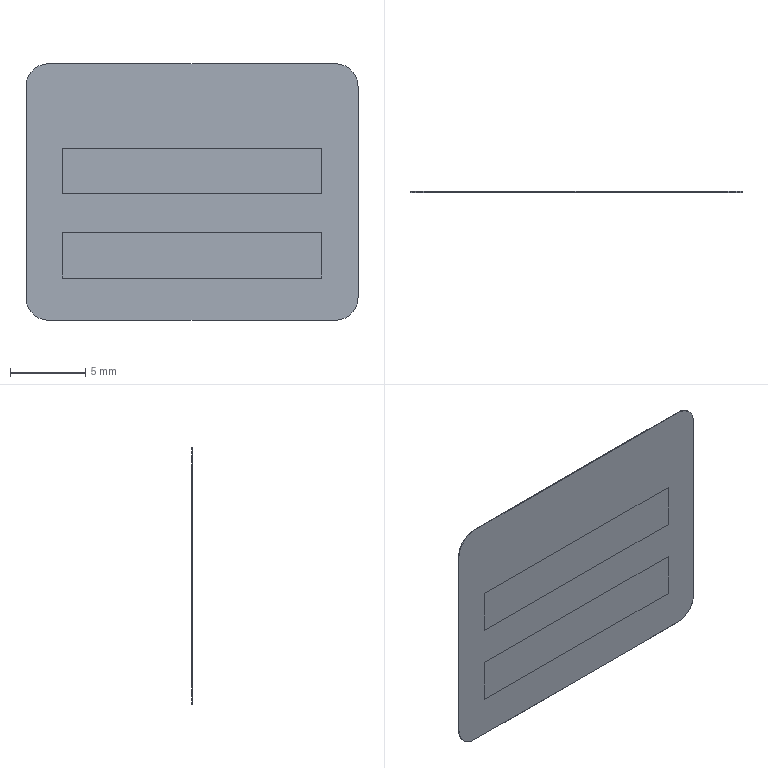Part | NX | features BREP 1 | 1 solid | 12 faces | box 22 x 0.06 x 17 mm | volume 18.947 mm3 | plane 8 | cylinder 4 | commonest cylinder face diameters 3 x4
STEP:
#1=CARTESIAN_POINT('',(2.4,-0.005,2.8));
#2=VERTEX_POINT('',#1);
#3=CARTESIAN_POINT('',(19.6,-0.005,2.8));
#4=VERTEX_POINT('',#3);
#5=CARTESIAN_POINT('',(2.4,-0.01,2.8));
#6=CARTESIAN_POINT('',(8.133,-0.01,2.8));
#7=CARTESIAN_POINT('',(13.867,-0.01,2.8));
#8=CARTESIAN_POINT('',(19.6,-0.01,2.8));
#9=B_SPLINE_CURVE_WITH_KNOTS('',3,(#5,#6,#7,#8),.UNSPECIFIED.,.F.,.F.,(4,4),(0.,1.),.UNSPECIFIED.);
#10=EDGE_CURVE('',#2,#4,#9,.T.);
#11=ORIENTED_EDGE('',*,*,#10,.T.);
#12=CARTESIAN_POINT('',(19.6,-0.005,5.8));
#13=VERTEX_POINT('',#12);
#14=CARTESIAN_POINT('',(19.6,-0.01,2.8));
#15=CARTESIAN_POINT('',(19.6,-0.01,3.8));
#16=CARTESIAN_POINT('',(19.6,-0.01,4.8));
#17=CARTESIAN_POINT('',(19.6,-0.01,5.8));
#18=B_SPLINE_CURVE_WITH_KNOTS('',3,(#14,#15,#16,#17),.UNSPECIFIED.,.F.,.F.,(4,4),(0.,1.),.UNSPECIFIED.);
#19=EDGE_CURVE('',#4,#13,#18,.T.);
#20=ORIENTED_EDGE('',*,*,#19,.T.);
#21=CARTESIAN_POINT('',(2.4,-0.005,5.8));
#22=VERTEX_POINT('',#21);
#23=CARTESIAN_POINT('',(19.6,-0.01,5.8));
#24=CARTESIAN_POINT('',(13.867,-0.01,5.8));
#25=CARTESIAN_POINT('',(8.133,-0.01,5.8));
#26=CARTESIAN_POINT('',(2.4,-0.01,5.8));
#27=B_SPLINE_CURVE_WITH_KNOTS('',3,(#23,#24,#25,#26),.UNSPECIFIED.,.F.,.F.,(4,4),(0.,1.),.UNSPECIFIED.);
#28=EDGE_CURVE('',#13,#22,#27,.T.);
#29=ORIENTED_EDGE('',*,*,#28,.T.);
#30=CARTESIAN_POINT('',(2.4,-0.01,5.8));
#31=CARTESIAN_POINT('',(2.4,-0.01,4.8));
#32=CARTESIAN_POINT('',(2.4,-0.01,3.8));
#33=CARTESIAN_POINT('',(2.4,-0.01,2.8));
#34=B_SPLINE_CURVE_WITH_KNOTS('',3,(#30,#31,#32,#33),.UNSPECIFIED.,.F.,.F.,(4,4),(0.,1.),.UNSPECIFIED.);
#35=EDGE_CURVE('',#22,#2,#34,.T.);
#36=ORIENTED_EDGE('',*,*,#35,.T.);
#37=EDGE_LOOP('',(#11,#20,#29,#36));
#38=FACE_BOUND('',#37,.T.);
#39=CARTESIAN_POINT('',(2.4,-0.01,2.8));
#40=DIRECTION('',(0.,-1.,0.));
#41=DIRECTION('',(0.,0.,1.));
#42=AXIS2_PLACEMENT_3D('',#39,#40,#41);
#43=PLANE('',#42);
#44=ADVANCED_FACE('',(#38),#43,.T.);
#45=CARTESIAN_POINT('',(2.4,-0.005,11.4));
#46=VERTEX_POINT('',#45);
#47=CARTESIAN_POINT('',(2.4,-0.005,8.4));
#48=VERTEX_POINT('',#47);
#49=CARTESIAN_POINT('',(2.4,-0.01,11.4));
#50=CARTESIAN_POINT('',(2.4,-0.01,10.4));
#51=CARTESIAN_POINT('',(2.4,-0.01,9.4));
#52=CARTESIAN_POINT('',(2.4,-0.01,8.4));
#53=B_SPLINE_CURVE_WITH_KNOTS('',3,(#49,#50,#51,#52),.UNSPECIFIED.,.F.,.F.,(4,4),(0.,1.),.UNSPECIFIED.);
#54=EDGE_CURVE('',#46,#48,#53,.T.);
#55=ORIENTED_EDGE('',*,*,#54,.T.);
#56=CARTESIAN_POINT('',(19.6,-0.005,8.4));
#57=VERTEX_POINT('',#56);
#58=CARTESIAN_POINT('',(2.4,-0.01,8.4));
#59=CARTESIAN_POINT('',(8.133,-0.01,8.4));
#60=CARTESIAN_POINT('',(13.867,-0.01,8.4));
#61=CARTESIAN_POINT('',(19.6,-0.01,8.4));
#62=B_SPLINE_CURVE_WITH_KNOTS('',3,(#58,#59,#60,#61),.UNSPECIFIED.,.F.,.F.,(4,4),(0.,1.),.UNSPECIFIED.);
#63=EDGE_CURVE('',#48,#57,#62,.T.);
#64=ORIENTED_EDGE('',*,*,#63,.T.);
#65=CARTESIAN_POINT('',(19.6,-0.005,11.4));
#66=VERTEX_POINT('',#65);
#67=CARTESIAN_POINT('',(19.6,-0.01,8.4));
#68=CARTESIAN_POINT('',(19.6,-0.01,9.4));
#69=CARTESIAN_POINT('',(19.6,-0.01,10.4));
#70=CARTESIAN_POINT('',(19.6,-0.01,11.4));
#71=B_SPLINE_CURVE_WITH_KNOTS('',3,(#67,#68,#69,#70),.UNSPECIFIED.,.F.,.F.,(4,4),(0.,1.),.UNSPECIFIED.);
#72=EDGE_CURVE('',#57,#66,#71,.T.);
#73=ORIENTED_EDGE('',*,*,#72,.T.);
#74=CARTESIAN_POINT('',(19.6,-0.01,11.4));
#75=CARTESIAN_POINT('',(13.867,-0.01,11.4));
#76=CARTESIAN_POINT('',(8.133,-0.01,11.4));
#77=CARTESIAN_POINT('',(2.4,-0.01,11.4));
#78=B_SPLINE_CURVE_WITH_KNOTS('',3,(#74,#75,#76,#77),.UNSPECIFIED.,.F.,.F.,(4,4),(0.,1.),.UNSPECIFIED.);
#79=EDGE_CURVE('',#66,#46,#78,.T.);
#80=ORIENTED_EDGE('',*,*,#79,.T.);
#81=EDGE_LOOP('',(#55,#64,#73,#80));
#82=FACE_BOUND('',#81,.T.);
#83=CARTESIAN_POINT('',(2.4,-0.01,8.4));
#84=DIRECTION('',(0.,-1.,0.));
#85=DIRECTION('',(0.,0.,1.));
#86=AXIS2_PLACEMENT_3D('',#83,#84,#85);
#87=PLANE('',#86);
#88=ADVANCED_FACE('',(#82),#87,.T.);
#89=CARTESIAN_POINT('',(1.5,0.,0.));
#90=VERTEX_POINT('',#89);
#91=CARTESIAN_POINT('',(20.5,0.,0.));
#92=VERTEX_POINT('',#91);
#93=CARTESIAN_POINT('',(1.5,0.,0.));
#94=DIRECTION('',(1.,0.,0.));
#95=VECTOR('',#94,1000.);
#96=LINE('',#93,#95);
#97=EDGE_CURVE('',#90,#92,#96,.T.);
#98=ORIENTED_EDGE('',*,*,#97,.T.);
#99=CARTESIAN_POINT('',(22.,0.,1.5));
#100=VERTEX_POINT('',#99);
#101=CARTESIAN_POINT('',(20.5,0.,1.5));
#102=DIRECTION('',(0.,-1.,0.));
#103=DIRECTION('',(0.,0.,-1.));
#104=AXIS2_PLACEMENT_3D('',#101,#102,#103);
#105=CIRCLE('',#104,1.5);
#106=EDGE_CURVE('',#92,#100,#105,.T.);
#107=ORIENTED_EDGE('',*,*,#106,.T.);
#108=CARTESIAN_POINT('',(22.,0.,15.5));
#109=VERTEX_POINT('',#108);
#110=CARTESIAN_POINT('',(22.,0.,1.5));
#111=DIRECTION('',(0.,0.,1.));
#112=VECTOR('',#111,1000.);
#113=LINE('',#110,#112);
#114=EDGE_CURVE('',#100,#109,#113,.T.);
#115=ORIENTED_EDGE('',*,*,#114,.T.);
#116=CARTESIAN_POINT('',(20.5,0.,17.));
#117=VERTEX_POINT('',#116);
#118=CARTESIAN_POINT('',(20.5,0.,15.5));
#119=DIRECTION('',(0.,-1.,0.));
#120=DIRECTION('',(1.,0.,0.));
#121=AXIS2_PLACEMENT_3D('',#118,#119,#120);
#122=CIRCLE('',#121,1.5);
#123=EDGE_CURVE('',#109,#117,#122,.T.);
#124=ORIENTED_EDGE('',*,*,#123,.T.);
#125=CARTESIAN_POINT('',(1.5,0.,17.));
#126=VERTEX_POINT('',#125);
#127=CARTESIAN_POINT('',(20.5,0.,17.));
#128=DIRECTION('',(-1.,0.,0.));
#129=VECTOR('',#128,1000.);
#130=LINE('',#127,#129);
#131=EDGE_CURVE('',#117,#126,#130,.T.);
#132=ORIENTED_EDGE('',*,*,#131,.T.);
#133=CARTESIAN_POINT('',(0.,0.,15.5));
#134=VERTEX_POINT('',#133);
#135=CARTESIAN_POINT('',(1.5,0.,15.5));
#136=DIRECTION('',(0.,-1.,0.));
#137=DIRECTION('',(0.,0.,1.));
#138=AXIS2_PLACEMENT_3D('',#135,#136,#137);
#139=CIRCLE('',#138,1.5);
#140=EDGE_CURVE('',#126,#134,#139,.T.);
#141=ORIENTED_EDGE('',*,*,#140,.T.);
#142=CARTESIAN_POINT('',(0.,0.,1.5));
#143=VERTEX_POINT('',#142);
#144=CARTESIAN_POINT('',(0.,0.,15.5));
#145=DIRECTION('',(0.,0.,-1.));
#146=VECTOR('',#145,1000.);
#147=LINE('',#144,#146);
#148=EDGE_CURVE('',#134,#143,#147,.T.);
#149=ORIENTED_EDGE('',*,*,#148,.T.);
#150=CARTESIAN_POINT('',(1.5,0.,1.5));
#151=DIRECTION('',(0.,-1.,0.));
#152=DIRECTION('',(-1.,0.,0.));
#153=AXIS2_PLACEMENT_3D('',#150,#151,#152);
#154=CIRCLE('',#153,1.5);
#155=EDGE_CURVE('',#143,#90,#154,.T.);
#156=ORIENTED_EDGE('',*,*,#155,.T.);
#157=EDGE_LOOP('',(#98,#107,#115,#124,#132,#141,#149,#156));
#158=FACE_BOUND('',#157,.T.);
#159=ORIENTED_EDGE('',*,*,#28,.F.);
#160=ORIENTED_EDGE('',*,*,#19,.F.);
#161=ORIENTED_EDGE('',*,*,#10,.F.);
#162=ORIENTED_EDGE('',*,*,#35,.F.);
#163=EDGE_LOOP('',(#159,#160,#161,#162));
#164=FACE_BOUND('',#163,.T.);
#165=ORIENTED_EDGE('',*,*,#72,.F.);
#166=ORIENTED_EDGE('',*,*,#63,.F.);
#167=ORIENTED_EDGE('',*,*,#54,.F.);
#168=ORIENTED_EDGE('',*,*,#79,.F.);
#169=EDGE_LOOP('',(#165,#166,#167,#168));
#170=FACE_BOUND('',#169,.T.);
#171=CARTESIAN_POINT('',(0.,0.,0.));
#172=DIRECTION('',(0.,-1.,0.));
#173=DIRECTION('',(0.,0.,1.));
#174=AXIS2_PLACEMENT_3D('',#171,#172,#173);
#175=PLANE('',#174);
#176=ADVANCED_FACE('',(#158,#164,#170),#175,.T.);
#177=CARTESIAN_POINT('',(1.5,0.05,0.));
#178=VERTEX_POINT('',#177);
#179=CARTESIAN_POINT('',(20.5,0.05,0.));
#180=VERTEX_POINT('',#179);
#181=CARTESIAN_POINT('',(1.5,0.05,0.));
#182=DIRECTION('',(1.,0.,0.));
#183=VECTOR('',#182,1000.);
#184=LINE('',#181,#183);
#185=EDGE_CURVE('',#178,#180,#184,.T.);
#186=ORIENTED_EDGE('',*,*,#185,.F.);
#187=CARTESIAN_POINT('',(0.,0.05,1.5));
#188=VERTEX_POINT('',#187);
#189=CARTESIAN_POINT('',(1.5,0.05,1.5));
#190=DIRECTION('',(0.,-1.,0.));
#191=DIRECTION('',(-1.,0.,0.));
#192=AXIS2_PLACEMENT_3D('',#189,#190,#191);
#193=CIRCLE('',#192,1.5);
#194=EDGE_CURVE('',#188,#178,#193,.T.);
#195=ORIENTED_EDGE('',*,*,#194,.F.);
#196=CARTESIAN_POINT('',(0.,0.05,15.5));
#197=VERTEX_POINT('',#196);
#198=CARTESIAN_POINT('',(0.,0.05,15.5));
#199=DIRECTION('',(0.,0.,-1.));
#200=VECTOR('',#199,1000.);
#201=LINE('',#198,#200);
#202=EDGE_CURVE('',#197,#188,#201,.T.);
#203=ORIENTED_EDGE('',*,*,#202,.F.);
#204=CARTESIAN_POINT('',(1.5,0.05,17.));
#205=VERTEX_POINT('',#204);
#206=CARTESIAN_POINT('',(1.5,0.05,15.5));
#207=DIRECTION('',(0.,-1.,0.));
#208=DIRECTION('',(0.,0.,1.));
#209=AXIS2_PLACEMENT_3D('',#206,#207,#208);
#210=CIRCLE('',#209,1.5);
#211=EDGE_CURVE('',#205,#197,#210,.T.);
#212=ORIENTED_EDGE('',*,*,#211,.F.);
#213=CARTESIAN_POINT('',(20.5,0.05,17.));
#214=VERTEX_POINT('',#213);
#215=CARTESIAN_POINT('',(20.5,0.05,17.));
#216=DIRECTION('',(-1.,0.,0.));
#217=VECTOR('',#216,1000.);
#218=LINE('',#215,#217);
#219=EDGE_CURVE('',#214,#205,#218,.T.);
#220=ORIENTED_EDGE('',*,*,#219,.F.);
#221=CARTESIAN_POINT('',(22.,0.05,15.5));
#222=VERTEX_POINT('',#221);
#223=CARTESIAN_POINT('',(20.5,0.05,15.5));
#224=DIRECTION('',(0.,-1.,0.));
#225=DIRECTION('',(1.,0.,0.));
#226=AXIS2_PLACEMENT_3D('',#223,#224,#225);
#227=CIRCLE('',#226,1.5);
#228=EDGE_CURVE('',#222,#214,#227,.T.);
#229=ORIENTED_EDGE('',*,*,#228,.F.);
#230=CARTESIAN_POINT('',(22.,0.05,1.5));
#231=VERTEX_POINT('',#230);
#232=CARTESIAN_POINT('',(22.,0.05,1.5));
#233=DIRECTION('',(0.,0.,1.));
#234=VECTOR('',#233,1000.);
#235=LINE('',#232,#234);
#236=EDGE_CURVE('',#231,#222,#235,.T.);
#237=ORIENTED_EDGE('',*,*,#236,.F.);
#238=CARTESIAN_POINT('',(20.5,0.05,1.5));
#239=DIRECTION('',(0.,-1.,0.));
#240=DIRECTION('',(0.,0.,-1.));
#241=AXIS2_PLACEMENT_3D('',#238,#239,#240);
#242=CIRCLE('',#241,1.5);
#243=EDGE_CURVE('',#180,#231,#242,.T.);
#244=ORIENTED_EDGE('',*,*,#243,.F.);
#245=EDGE_LOOP('',(#186,#195,#203,#212,#220,#229,#237,#244));
#246=FACE_BOUND('',#245,.T.);
#247=CARTESIAN_POINT('',(0.,0.05,0.));
#248=DIRECTION('',(0.,1.,0.));
#249=DIRECTION('',(-1.,0.,0.));
#250=AXIS2_PLACEMENT_3D('',#247,#248,#249);
#251=PLANE('',#250);
#252=ADVANCED_FACE('',(#246),#251,.T.);
#253=ORIENTED_EDGE('',*,*,#194,.T.);
#254=CARTESIAN_POINT('',(1.5,0.,0.));
#255=DIRECTION('',(0.,1.,0.));
#256=VECTOR('',#255,1000.);
#257=LINE('',#254,#256);
#258=EDGE_CURVE('',#90,#178,#257,.T.);
#259=ORIENTED_EDGE('',*,*,#258,.F.);
#260=ORIENTED_EDGE('',*,*,#155,.F.);
#261=CARTESIAN_POINT('',(0.,0.,1.5));
#262=DIRECTION('',(0.,1.,0.));
#263=VECTOR('',#262,1000.);
#264=LINE('',#261,#263);
#265=EDGE_CURVE('',#143,#188,#264,.T.);
#266=ORIENTED_EDGE('',*,*,#265,.T.);
#267=EDGE_LOOP('',(#253,#259,#260,#266));
#268=FACE_BOUND('',#267,.T.);
#269=CARTESIAN_POINT('',(1.5,0.05,1.5));
#270=DIRECTION('',(0.,-1.,0.));
#271=DIRECTION('',(-0.7071,0.,-0.7071));
#272=AXIS2_PLACEMENT_3D('',#269,#270,#271);
#273=CYLINDRICAL_SURFACE('',#272,1.5);
#274=ADVANCED_FACE('',(#268),#273,.T.);
#275=CARTESIAN_POINT('',(0.,0.,15.5));
#276=DIRECTION('',(0.,1.,0.));
#277=VECTOR('',#276,1000.);
#278=LINE('',#275,#277);
#279=EDGE_CURVE('',#134,#197,#278,.T.);
#280=ORIENTED_EDGE('',*,*,#279,.T.);
#281=ORIENTED_EDGE('',*,*,#202,.T.);
#282=ORIENTED_EDGE('',*,*,#265,.F.);
#283=ORIENTED_EDGE('',*,*,#148,.F.);
#284=EDGE_LOOP('',(#280,#281,#282,#283));
#285=FACE_BOUND('',#284,.T.);
#286=CARTESIAN_POINT('',(0.,0.,15.5));
#287=DIRECTION('',(-1.,0.,0.));
#288=DIRECTION('',(0.,0.,-1.));
#289=AXIS2_PLACEMENT_3D('',#286,#287,#288);
#290=PLANE('',#289);
#291=ADVANCED_FACE('',(#285),#290,.T.);
#292=ORIENTED_EDGE('',*,*,#211,.T.);
#293=ORIENTED_EDGE('',*,*,#279,.F.);
#294=ORIENTED_EDGE('',*,*,#140,.F.);
#295=CARTESIAN_POINT('',(1.5,0.,17.));
#296=DIRECTION('',(0.,1.,0.));
#297=VECTOR('',#296,1000.);
#298=LINE('',#295,#297);
#299=EDGE_CURVE('',#126,#205,#298,.T.);
#300=ORIENTED_EDGE('',*,*,#299,.T.);
#301=EDGE_LOOP('',(#292,#293,#294,#300));
#302=FACE_BOUND('',#301,.T.);
#303=CARTESIAN_POINT('',(1.5,0.05,15.5));
#304=DIRECTION('',(0.,-1.,0.));
#305=DIRECTION('',(-0.7071,0.,0.7071));
#306=AXIS2_PLACEMENT_3D('',#303,#304,#305);
#307=CYLINDRICAL_SURFACE('',#306,1.5);
#308=ADVANCED_FACE('',(#302),#307,.T.);
#309=CARTESIAN_POINT('',(20.5,0.,17.));
#310=DIRECTION('',(0.,1.,0.));
#311=VECTOR('',#310,1000.);
#312=LINE('',#309,#311);
#313=EDGE_CURVE('',#117,#214,#312,.T.);
#314=ORIENTED_EDGE('',*,*,#313,.T.);
#315=ORIENTED_EDGE('',*,*,#219,.T.);
#316=ORIENTED_EDGE('',*,*,#299,.F.);
#317=ORIENTED_EDGE('',*,*,#131,.F.);
#318=EDGE_LOOP('',(#314,#315,#316,#317));
#319=FACE_BOUND('',#318,.T.);
#320=CARTESIAN_POINT('',(20.5,0.,17.));
#321=DIRECTION('',(0.,0.,1.));
#322=DIRECTION('',(-1.,0.,0.));
#323=AXIS2_PLACEMENT_3D('',#320,#321,#322);
#324=PLANE('',#323);
#325=ADVANCED_FACE('',(#319),#324,.T.);
#326=ORIENTED_EDGE('',*,*,#228,.T.);
#327=ORIENTED_EDGE('',*,*,#313,.F.);
#328=ORIENTED_EDGE('',*,*,#123,.F.);
#329=CARTESIAN_POINT('',(22.,0.,15.5));
#330=DIRECTION('',(0.,1.,0.));
#331=VECTOR('',#330,1000.);
#332=LINE('',#329,#331);
#333=EDGE_CURVE('',#109,#222,#332,.T.);
#334=ORIENTED_EDGE('',*,*,#333,.T.);
#335=EDGE_LOOP('',(#326,#327,#328,#334));
#336=FACE_BOUND('',#335,.T.);
#337=CARTESIAN_POINT('',(20.5,0.05,15.5));
#338=DIRECTION('',(0.,-1.,0.));
#339=DIRECTION('',(0.7071,0.,0.7071));
#340=AXIS2_PLACEMENT_3D('',#337,#338,#339);
#341=CYLINDRICAL_SURFACE('',#340,1.5);
#342=ADVANCED_FACE('',(#336),#341,.T.);
#343=CARTESIAN_POINT('',(22.,0.,1.5));
#344=DIRECTION('',(0.,1.,0.));
#345=VECTOR('',#344,1000.);
#346=LINE('',#343,#345);
#347=EDGE_CURVE('',#100,#231,#346,.T.);
#348=ORIENTED_EDGE('',*,*,#347,.T.);
#349=ORIENTED_EDGE('',*,*,#236,.T.);
#350=ORIENTED_EDGE('',*,*,#333,.F.);
#351=ORIENTED_EDGE('',*,*,#114,.F.);
#352=EDGE_LOOP('',(#348,#349,#350,#351));
#353=FACE_BOUND('',#352,.T.);
#354=CARTESIAN_POINT('',(22.,0.,1.5));
#355=DIRECTION('',(1.,0.,0.));
#356=DIRECTION('',(0.,-1.,0.));
#357=AXIS2_PLACEMENT_3D('',#354,#355,#356);
#358=PLANE('',#357);
#359=ADVANCED_FACE('',(#353),#358,.T.);
#360=ORIENTED_EDGE('',*,*,#243,.T.);
#361=ORIENTED_EDGE('',*,*,#347,.F.);
#362=ORIENTED_EDGE('',*,*,#106,.F.);
#363=CARTESIAN_POINT('',(20.5,0.,0.));
#364=DIRECTION('',(0.,1.,0.));
#365=VECTOR('',#364,1000.);
#366=LINE('',#363,#365);
#367=EDGE_CURVE('',#92,#180,#366,.T.);
#368=ORIENTED_EDGE('',*,*,#367,.T.);
#369=EDGE_LOOP('',(#360,#361,#362,#368));
#370=FACE_BOUND('',#369,.T.);
#371=CARTESIAN_POINT('',(20.5,0.05,1.5));
#372=DIRECTION('',(0.,-1.,0.));
#373=DIRECTION('',(0.7071,0.,-0.7071));
#374=AXIS2_PLACEMENT_3D('',#371,#372,#373);
#375=CYLINDRICAL_SURFACE('',#374,1.5);
#376=ADVANCED_FACE('',(#370),#375,.T.);
#377=ORIENTED_EDGE('',*,*,#258,.T.);
#378=ORIENTED_EDGE('',*,*,#185,.T.);
#379=ORIENTED_EDGE('',*,*,#367,.F.);
#380=ORIENTED_EDGE('',*,*,#97,.F.);
#381=EDGE_LOOP('',(#377,#378,#379,#380));
#382=FACE_BOUND('',#381,.T.);
#383=CARTESIAN_POINT('',(1.5,0.,0.));
#384=DIRECTION('',(0.,0.,-1.));
#385=DIRECTION('',(0.,1.,0.));
#386=AXIS2_PLACEMENT_3D('',#383,#384,#385);
#387=PLANE('',#386);
#388=ADVANCED_FACE('',(#382),#387,.T.);
#389=CLOSED_SHELL('',(#44,#88,#176,#252,#274,#291,#308,#325,#342,#359,#376,#388));
#390=MANIFOLD_SOLID_BREP('',#389);
#391=(LENGTH_UNIT()NAMED_UNIT(*)SI_UNIT(.MILLI.,.METRE.));
#392=UNCERTAINTY_MEASURE_WITH_UNIT(LENGTH_MEASURE(0.0525),#391,'','');
#393=(NAMED_UNIT(*)PLANE_ANGLE_UNIT()SI_UNIT($,.RADIAN.));
#394=(NAMED_UNIT(*)SI_UNIT($,.STERADIAN.)SOLID_ANGLE_UNIT());
#395=(GEOMETRIC_REPRESENTATION_CONTEXT(3)GLOBAL_UNCERTAINTY_ASSIGNED_CONTEXT((#392))GLOBAL_UNIT_ASSIGNED_CONTEXT((#391,#393,#394))REPRESENTATION_CONTEXT('',''));
#396=ADVANCED_BREP_SHAPE_REPRESENTATION('',(#390),#395);